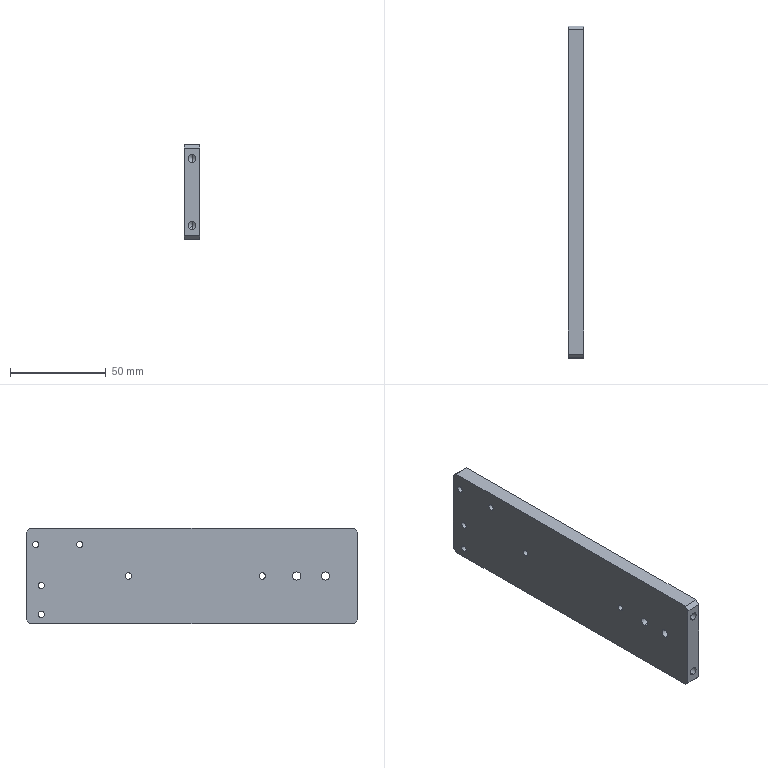Part | STEP file | FBDS-TL-001 | 1 solid | 34 faces | box 8 x 173.5 x 50 mm | volume 68338 mm3 | cylinder 20 | plane 10 | cone 4 | commonest cylinder face diameters 3.3 x12 4.2 x4 4.3 x4
STEP:
#1=CARTESIAN_POINT('',(0.,32.,27.15));
#2=VERTEX_POINT('',#1);
#3=CARTESIAN_POINT('',(0.,32.,22.85));
#4=VERTEX_POINT('',#3);
#5=CARTESIAN_POINT('',(0.,32.,25.));
#6=DIRECTION('',(1.,0.,0.));
#7=DIRECTION('',(0.,0.,-1.));
#8=AXIS2_PLACEMENT_3D('',#5,#6,#7);
#9=CIRCLE('',#8,2.15);
#10=EDGE_CURVE('',#2,#4,#9,.T.);
#11=ORIENTED_EDGE('',*,*,#10,.F.);
#12=CARTESIAN_POINT('',(8.,32.,27.15));
#13=VERTEX_POINT('',#12);
#14=CARTESIAN_POINT('',(8.,32.,27.15));
#15=DIRECTION('',(1.,0.,0.));
#16=VECTOR('',#15,1000.);
#17=LINE('',#14,#16);
#18=EDGE_CURVE('',#2,#13,#17,.T.);
#19=ORIENTED_EDGE('',*,*,#18,.T.);
#20=CARTESIAN_POINT('',(8.,32.,22.85));
#21=VERTEX_POINT('',#20);
#22=CARTESIAN_POINT('',(8.,32.,25.));
#23=DIRECTION('',(1.,0.,0.));
#24=DIRECTION('',(0.,0.,-1.));
#25=AXIS2_PLACEMENT_3D('',#22,#23,#24);
#26=CIRCLE('',#25,2.15);
#27=EDGE_CURVE('',#13,#21,#26,.T.);
#28=ORIENTED_EDGE('',*,*,#27,.T.);
#29=CARTESIAN_POINT('',(8.,32.,22.85));
#30=DIRECTION('',(1.,0.,0.));
#31=VECTOR('',#30,1000.);
#32=LINE('',#29,#31);
#33=EDGE_CURVE('',#4,#21,#32,.T.);
#34=ORIENTED_EDGE('',*,*,#33,.F.);
#35=EDGE_LOOP('',(#11,#19,#28,#34));
#36=FACE_OUTER_BOUND('',#35,.T.);
#37=CARTESIAN_POINT('',(8.,32.,25.));
#38=DIRECTION('',(1.,0.,0.));
#39=DIRECTION('',(0.,0.,-1.));
#40=AXIS2_PLACEMENT_3D('',#37,#38,#39);
#41=CYLINDRICAL_SURFACE('',#40,2.15);
#42=ADVANCED_FACE('',(#36),#41,.F.);
#43=CARTESIAN_POINT('',(0.,17.,27.15));
#44=VERTEX_POINT('',#43);
#45=CARTESIAN_POINT('',(0.,17.,22.85));
#46=VERTEX_POINT('',#45);
#47=CARTESIAN_POINT('',(0.,17.,25.));
#48=DIRECTION('',(1.,0.,0.));
#49=DIRECTION('',(0.,0.,-1.));
#50=AXIS2_PLACEMENT_3D('',#47,#48,#49);
#51=CIRCLE('',#50,2.15);
#52=EDGE_CURVE('',#44,#46,#51,.T.);
#53=ORIENTED_EDGE('',*,*,#52,.F.);
#54=CARTESIAN_POINT('',(8.,17.,27.15));
#55=VERTEX_POINT('',#54);
#56=CARTESIAN_POINT('',(8.,17.,27.15));
#57=DIRECTION('',(1.,0.,0.));
#58=VECTOR('',#57,1000.);
#59=LINE('',#56,#58);
#60=EDGE_CURVE('',#44,#55,#59,.T.);
#61=ORIENTED_EDGE('',*,*,#60,.T.);
#62=CARTESIAN_POINT('',(8.,17.,22.85));
#63=VERTEX_POINT('',#62);
#64=CARTESIAN_POINT('',(8.,17.,25.));
#65=DIRECTION('',(1.,0.,0.));
#66=DIRECTION('',(0.,0.,-1.));
#67=AXIS2_PLACEMENT_3D('',#64,#65,#66);
#68=CIRCLE('',#67,2.15);
#69=EDGE_CURVE('',#55,#63,#68,.T.);
#70=ORIENTED_EDGE('',*,*,#69,.T.);
#71=CARTESIAN_POINT('',(8.,17.,22.85));
#72=DIRECTION('',(1.,0.,0.));
#73=VECTOR('',#72,1000.);
#74=LINE('',#71,#73);
#75=EDGE_CURVE('',#46,#63,#74,.T.);
#76=ORIENTED_EDGE('',*,*,#75,.F.);
#77=EDGE_LOOP('',(#53,#61,#70,#76));
#78=FACE_OUTER_BOUND('',#77,.T.);
#79=CARTESIAN_POINT('',(8.,17.,25.));
#80=DIRECTION('',(1.,0.,0.));
#81=DIRECTION('',(0.,0.,-1.));
#82=AXIS2_PLACEMENT_3D('',#79,#80,#81);
#83=CYLINDRICAL_SURFACE('',#82,2.15);
#84=ADVANCED_FACE('',(#78),#83,.F.);
#85=CARTESIAN_POINT('',(0.,120.,26.65));
#86=VERTEX_POINT('',#85);
#87=CARTESIAN_POINT('',(0.,120.,23.35));
#88=VERTEX_POINT('',#87);
#89=CARTESIAN_POINT('',(0.,120.,25.));
#90=DIRECTION('',(1.,0.,0.));
#91=DIRECTION('',(0.,0.,-1.));
#92=AXIS2_PLACEMENT_3D('',#89,#90,#91);
#93=CIRCLE('',#92,1.65);
#94=EDGE_CURVE('',#86,#88,#93,.T.);
#95=ORIENTED_EDGE('',*,*,#94,.F.);
#96=CARTESIAN_POINT('',(8.,120.,26.65));
#97=VERTEX_POINT('',#96);
#98=CARTESIAN_POINT('',(8.,120.,26.65));
#99=DIRECTION('',(1.,0.,0.));
#100=VECTOR('',#99,1000.);
#101=LINE('',#98,#100);
#102=EDGE_CURVE('',#86,#97,#101,.T.);
#103=ORIENTED_EDGE('',*,*,#102,.T.);
#104=CARTESIAN_POINT('',(8.,120.,23.35));
#105=VERTEX_POINT('',#104);
#106=CARTESIAN_POINT('',(8.,120.,25.));
#107=DIRECTION('',(1.,0.,0.));
#108=DIRECTION('',(0.,0.,-1.));
#109=AXIS2_PLACEMENT_3D('',#106,#107,#108);
#110=CIRCLE('',#109,1.65);
#111=EDGE_CURVE('',#97,#105,#110,.T.);
#112=ORIENTED_EDGE('',*,*,#111,.T.);
#113=CARTESIAN_POINT('',(8.,120.,23.35));
#114=DIRECTION('',(1.,0.,0.));
#115=VECTOR('',#114,1000.);
#116=LINE('',#113,#115);
#117=EDGE_CURVE('',#88,#105,#116,.T.);
#118=ORIENTED_EDGE('',*,*,#117,.F.);
#119=EDGE_LOOP('',(#95,#103,#112,#118));
#120=FACE_OUTER_BOUND('',#119,.T.);
#121=CARTESIAN_POINT('',(8.,120.,25.));
#122=DIRECTION('',(1.,0.,0.));
#123=DIRECTION('',(0.,0.,-1.));
#124=AXIS2_PLACEMENT_3D('',#121,#122,#123);
#125=CYLINDRICAL_SURFACE('',#124,1.65);
#126=ADVANCED_FACE('',(#120),#125,.F.);
#127=CARTESIAN_POINT('',(0.,50.,26.65));
#128=VERTEX_POINT('',#127);
#129=CARTESIAN_POINT('',(0.,50.,23.35));
#130=VERTEX_POINT('',#129);
#131=CARTESIAN_POINT('',(0.,50.,25.));
#132=DIRECTION('',(1.,0.,0.));
#133=DIRECTION('',(0.,0.,-1.));
#134=AXIS2_PLACEMENT_3D('',#131,#132,#133);
#135=CIRCLE('',#134,1.65);
#136=EDGE_CURVE('',#128,#130,#135,.T.);
#137=ORIENTED_EDGE('',*,*,#136,.F.);
#138=CARTESIAN_POINT('',(8.,50.,26.65));
#139=VERTEX_POINT('',#138);
#140=CARTESIAN_POINT('',(8.,50.,26.65));
#141=DIRECTION('',(1.,0.,0.));
#142=VECTOR('',#141,1000.);
#143=LINE('',#140,#142);
#144=EDGE_CURVE('',#128,#139,#143,.T.);
#145=ORIENTED_EDGE('',*,*,#144,.T.);
#146=CARTESIAN_POINT('',(8.,50.,23.35));
#147=VERTEX_POINT('',#146);
#148=CARTESIAN_POINT('',(8.,50.,25.));
#149=DIRECTION('',(1.,0.,0.));
#150=DIRECTION('',(0.,0.,-1.));
#151=AXIS2_PLACEMENT_3D('',#148,#149,#150);
#152=CIRCLE('',#151,1.65);
#153=EDGE_CURVE('',#139,#147,#152,.T.);
#154=ORIENTED_EDGE('',*,*,#153,.T.);
#155=CARTESIAN_POINT('',(8.,50.,23.35));
#156=DIRECTION('',(1.,0.,0.));
#157=VECTOR('',#156,1000.);
#158=LINE('',#155,#157);
#159=EDGE_CURVE('',#130,#147,#158,.T.);
#160=ORIENTED_EDGE('',*,*,#159,.F.);
#161=EDGE_LOOP('',(#137,#145,#154,#160));
#162=FACE_OUTER_BOUND('',#161,.T.);
#163=CARTESIAN_POINT('',(8.,50.,25.));
#164=DIRECTION('',(1.,0.,0.));
#165=DIRECTION('',(0.,0.,-1.));
#166=AXIS2_PLACEMENT_3D('',#163,#164,#165);
#167=CYLINDRICAL_SURFACE('',#166,1.65);
#168=ADVANCED_FACE('',(#162),#167,.F.);
#169=CARTESIAN_POINT('',(8.,165.5,18.35));
#170=VERTEX_POINT('',#169);
#171=CARTESIAN_POINT('',(8.,165.5,21.65));
#172=VERTEX_POINT('',#171);
#173=CARTESIAN_POINT('',(8.,165.5,20.));
#174=DIRECTION('',(-1.,0.,0.));
#175=DIRECTION('',(0.,-1.,0.));
#176=AXIS2_PLACEMENT_3D('',#173,#174,#175);
#177=CIRCLE('',#176,1.65);
#178=EDGE_CURVE('',#170,#172,#177,.T.);
#179=ORIENTED_EDGE('',*,*,#178,.F.);
#180=CARTESIAN_POINT('',(0.,165.5,18.35));
#181=VERTEX_POINT('',#180);
#182=CARTESIAN_POINT('',(0.,165.5,18.35));
#183=DIRECTION('',(-1.,0.,0.));
#184=VECTOR('',#183,1000.);
#185=LINE('',#182,#184);
#186=EDGE_CURVE('',#170,#181,#185,.T.);
#187=ORIENTED_EDGE('',*,*,#186,.T.);
#188=CARTESIAN_POINT('',(0.,165.5,21.65));
#189=VERTEX_POINT('',#188);
#190=CARTESIAN_POINT('',(0.,165.5,20.));
#191=DIRECTION('',(-1.,0.,0.));
#192=DIRECTION('',(0.,0.,1.));
#193=AXIS2_PLACEMENT_3D('',#190,#191,#192);
#194=CIRCLE('',#193,1.65);
#195=EDGE_CURVE('',#181,#189,#194,.T.);
#196=ORIENTED_EDGE('',*,*,#195,.T.);
#197=CARTESIAN_POINT('',(0.,165.5,21.65));
#198=DIRECTION('',(-1.,0.,0.));
#199=VECTOR('',#198,1000.);
#200=LINE('',#197,#199);
#201=EDGE_CURVE('',#172,#189,#200,.T.);
#202=ORIENTED_EDGE('',*,*,#201,.F.);
#203=EDGE_LOOP('',(#179,#187,#196,#202));
#204=FACE_OUTER_BOUND('',#203,.T.);
#205=CARTESIAN_POINT('',(0.,165.5,20.));
#206=DIRECTION('',(-1.,0.,0.));
#207=DIRECTION('',(0.,0.,1.));
#208=AXIS2_PLACEMENT_3D('',#205,#206,#207);
#209=CYLINDRICAL_SURFACE('',#208,1.65);
#210=ADVANCED_FACE('',(#204),#209,.F.);
#211=CARTESIAN_POINT('',(8.,165.5,3.35));
#212=VERTEX_POINT('',#211);
#213=CARTESIAN_POINT('',(8.,165.5,6.65));
#214=VERTEX_POINT('',#213);
#215=CARTESIAN_POINT('',(8.,165.5,5.));
#216=DIRECTION('',(-1.,0.,0.));
#217=DIRECTION('',(0.,-1.,0.));
#218=AXIS2_PLACEMENT_3D('',#215,#216,#217);
#219=CIRCLE('',#218,1.65);
#220=EDGE_CURVE('',#212,#214,#219,.T.);
#221=ORIENTED_EDGE('',*,*,#220,.F.);
#222=CARTESIAN_POINT('',(0.,165.5,3.35));
#223=VERTEX_POINT('',#222);
#224=CARTESIAN_POINT('',(0.,165.5,3.35));
#225=DIRECTION('',(-1.,0.,0.));
#226=VECTOR('',#225,1000.);
#227=LINE('',#224,#226);
#228=EDGE_CURVE('',#212,#223,#227,.T.);
#229=ORIENTED_EDGE('',*,*,#228,.T.);
#230=CARTESIAN_POINT('',(0.,165.5,6.65));
#231=VERTEX_POINT('',#230);
#232=CARTESIAN_POINT('',(0.,165.5,5.));
#233=DIRECTION('',(-1.,0.,0.));
#234=DIRECTION('',(0.,0.,1.));
#235=AXIS2_PLACEMENT_3D('',#232,#233,#234);
#236=CIRCLE('',#235,1.65);
#237=EDGE_CURVE('',#223,#231,#236,.T.);
#238=ORIENTED_EDGE('',*,*,#237,.T.);
#239=CARTESIAN_POINT('',(0.,165.5,6.65));
#240=DIRECTION('',(-1.,0.,0.));
#241=VECTOR('',#240,1000.);
#242=LINE('',#239,#241);
#243=EDGE_CURVE('',#214,#231,#242,.T.);
#244=ORIENTED_EDGE('',*,*,#243,.F.);
#245=EDGE_LOOP('',(#221,#229,#238,#244));
#246=FACE_OUTER_BOUND('',#245,.T.);
#247=CARTESIAN_POINT('',(0.,165.5,5.));
#248=DIRECTION('',(-1.,0.,0.));
#249=DIRECTION('',(0.,0.,1.));
#250=AXIS2_PLACEMENT_3D('',#247,#248,#249);
#251=CYLINDRICAL_SURFACE('',#250,1.65);
#252=ADVANCED_FACE('',(#246),#251,.F.);
#253=CARTESIAN_POINT('',(4.,12.4,9.6));
#254=VERTEX_POINT('',#253);
#255=CARTESIAN_POINT('',(4.,12.4,5.4));
#256=VERTEX_POINT('',#255);
#257=CARTESIAN_POINT('',(4.,12.4,7.5));
#258=DIRECTION('',(0.,-1.,0.));
#259=DIRECTION('',(0.,0.,-1.));
#260=AXIS2_PLACEMENT_3D('',#257,#258,#259);
#261=CIRCLE('',#260,2.1);
#262=EDGE_CURVE('',#254,#256,#261,.T.);
#263=ORIENTED_EDGE('',*,*,#262,.F.);
#264=CARTESIAN_POINT('',(4.,0.,9.6));
#265=VERTEX_POINT('',#264);
#266=CARTESIAN_POINT('',(4.,0.,9.6));
#267=DIRECTION('',(0.,-1.,0.));
#268=VECTOR('',#267,1000.);
#269=LINE('',#266,#268);
#270=EDGE_CURVE('',#254,#265,#269,.T.);
#271=ORIENTED_EDGE('',*,*,#270,.T.);
#272=CARTESIAN_POINT('',(4.,0.,5.4));
#273=VERTEX_POINT('',#272);
#274=CARTESIAN_POINT('',(4.,0.,7.5));
#275=DIRECTION('',(0.,-1.,0.));
#276=DIRECTION('',(0.,0.,-1.));
#277=AXIS2_PLACEMENT_3D('',#274,#275,#276);
#278=CIRCLE('',#277,2.1);
#279=EDGE_CURVE('',#265,#273,#278,.T.);
#280=ORIENTED_EDGE('',*,*,#279,.T.);
#281=CARTESIAN_POINT('',(4.,0.,5.4));
#282=DIRECTION('',(0.,-1.,0.));
#283=VECTOR('',#282,1000.);
#284=LINE('',#281,#283);
#285=EDGE_CURVE('',#256,#273,#284,.T.);
#286=ORIENTED_EDGE('',*,*,#285,.F.);
#287=EDGE_LOOP('',(#263,#271,#280,#286));
#288=FACE_OUTER_BOUND('',#287,.T.);
#289=CARTESIAN_POINT('',(4.,0.,7.5));
#290=DIRECTION('',(0.,-1.,0.));
#291=DIRECTION('',(0.,0.,-1.));
#292=AXIS2_PLACEMENT_3D('',#289,#290,#291);
#293=CYLINDRICAL_SURFACE('',#292,2.1);
#294=ADVANCED_FACE('',(#288),#293,.F.);
#295=CARTESIAN_POINT('',(4.,13.662,7.5));
#296=VERTEX_POINT('',#295);
#297=CARTESIAN_POINT('',(4.,12.4,5.4));
#298=DIRECTION('',(0.,-0.515,-0.8572));
#299=VECTOR('',#298,1000.);
#300=LINE('',#297,#299);
#301=EDGE_CURVE('',#296,#256,#300,.T.);
#302=ORIENTED_EDGE('',*,*,#301,.F.);
#303=CARTESIAN_POINT('',(4.,12.4,9.6));
#304=DIRECTION('',(0.,-0.515,0.8572));
#305=VECTOR('',#304,1000.);
#306=LINE('',#303,#305);
#307=EDGE_CURVE('',#296,#254,#306,.T.);
#308=ORIENTED_EDGE('',*,*,#307,.T.);
#309=ORIENTED_EDGE('',*,*,#262,.T.);
#310=EDGE_LOOP('',(#302,#308,#309));
#311=FACE_OUTER_BOUND('',#310,.T.);
#312=CARTESIAN_POINT('',(4.,12.4,7.5));
#313=DIRECTION('',(0.,-1.,0.));
#314=DIRECTION('',(0.,0.,-1.));
#315=AXIS2_PLACEMENT_3D('',#312,#313,#314);
#316=CONICAL_SURFACE('',#315,2.1,1.03);
#317=ADVANCED_FACE('',(#311),#316,.F.);
#318=CARTESIAN_POINT('',(4.,12.4,44.6));
#319=VERTEX_POINT('',#318);
#320=CARTESIAN_POINT('',(4.,12.4,40.4));
#321=VERTEX_POINT('',#320);
#322=CARTESIAN_POINT('',(4.,12.4,42.5));
#323=DIRECTION('',(0.,-1.,0.));
#324=DIRECTION('',(0.,0.,-1.));
#325=AXIS2_PLACEMENT_3D('',#322,#323,#324);
#326=CIRCLE('',#325,2.1);
#327=EDGE_CURVE('',#319,#321,#326,.T.);
#328=ORIENTED_EDGE('',*,*,#327,.F.);
#329=CARTESIAN_POINT('',(4.,0.,44.6));
#330=VERTEX_POINT('',#329);
#331=CARTESIAN_POINT('',(4.,0.,44.6));
#332=DIRECTION('',(0.,-1.,0.));
#333=VECTOR('',#332,1000.);
#334=LINE('',#331,#333);
#335=EDGE_CURVE('',#319,#330,#334,.T.);
#336=ORIENTED_EDGE('',*,*,#335,.T.);
#337=CARTESIAN_POINT('',(4.,0.,40.4));
#338=VERTEX_POINT('',#337);
#339=CARTESIAN_POINT('',(4.,0.,42.5));
#340=DIRECTION('',(0.,-1.,0.));
#341=DIRECTION('',(0.,0.,-1.));
#342=AXIS2_PLACEMENT_3D('',#339,#340,#341);
#343=CIRCLE('',#342,2.1);
#344=EDGE_CURVE('',#330,#338,#343,.T.);
#345=ORIENTED_EDGE('',*,*,#344,.T.);
#346=CARTESIAN_POINT('',(4.,0.,40.4));
#347=DIRECTION('',(0.,-1.,0.));
#348=VECTOR('',#347,1000.);
#349=LINE('',#346,#348);
#350=EDGE_CURVE('',#321,#338,#349,.T.);
#351=ORIENTED_EDGE('',*,*,#350,.F.);
#352=EDGE_LOOP('',(#328,#336,#345,#351));
#353=FACE_OUTER_BOUND('',#352,.T.);
#354=CARTESIAN_POINT('',(4.,0.,42.5));
#355=DIRECTION('',(0.,-1.,0.));
#356=DIRECTION('',(0.,0.,-1.));
#357=AXIS2_PLACEMENT_3D('',#354,#355,#356);
#358=CYLINDRICAL_SURFACE('',#357,2.1);
#359=ADVANCED_FACE('',(#353),#358,.F.);
#360=CARTESIAN_POINT('',(4.,13.662,42.5));
#361=VERTEX_POINT('',#360);
#362=CARTESIAN_POINT('',(4.,12.4,40.4));
#363=DIRECTION('',(0.,-0.515,-0.8572));
#364=VECTOR('',#363,1000.);
#365=LINE('',#362,#364);
#366=EDGE_CURVE('',#361,#321,#365,.T.);
#367=ORIENTED_EDGE('',*,*,#366,.F.);
#368=CARTESIAN_POINT('',(4.,12.4,44.6));
#369=DIRECTION('',(0.,-0.515,0.8572));
#370=VECTOR('',#369,1000.);
#371=LINE('',#368,#370);
#372=EDGE_CURVE('',#361,#319,#371,.T.);
#373=ORIENTED_EDGE('',*,*,#372,.T.);
#374=ORIENTED_EDGE('',*,*,#327,.T.);
#375=EDGE_LOOP('',(#367,#373,#374));
#376=FACE_OUTER_BOUND('',#375,.T.);
#377=CARTESIAN_POINT('',(4.,12.4,42.5));
#378=DIRECTION('',(0.,-1.,0.));
#379=DIRECTION('',(0.,0.,-1.));
#380=AXIS2_PLACEMENT_3D('',#377,#378,#379);
#381=CONICAL_SURFACE('',#380,2.1,1.03);
#382=ADVANCED_FACE('',(#376),#381,.F.);
#383=CARTESIAN_POINT('',(0.,168.5,43.15));
#384=VERTEX_POINT('',#383);
#385=CARTESIAN_POINT('',(0.,168.5,39.85));
#386=VERTEX_POINT('',#385);
#387=CARTESIAN_POINT('',(0.,168.5,41.5));
#388=DIRECTION('',(1.,0.,0.));
#389=DIRECTION('',(0.,0.,-1.));
#390=AXIS2_PLACEMENT_3D('',#387,#388,#389);
#391=CIRCLE('',#390,1.65);
#392=EDGE_CURVE('',#384,#386,#391,.T.);
#393=ORIENTED_EDGE('',*,*,#392,.F.);
#394=CARTESIAN_POINT('',(8.,168.5,43.15));
#395=VERTEX_POINT('',#394);
#396=CARTESIAN_POINT('',(8.,168.5,43.15));
#397=DIRECTION('',(1.,0.,0.));
#398=VECTOR('',#397,1000.);
#399=LINE('',#396,#398);
#400=EDGE_CURVE('',#384,#395,#399,.T.);
#401=ORIENTED_EDGE('',*,*,#400,.T.);
#402=CARTESIAN_POINT('',(8.,168.5,39.85));
#403=VERTEX_POINT('',#402);
#404=CARTESIAN_POINT('',(8.,168.5,41.5));
#405=DIRECTION('',(1.,0.,0.));
#406=DIRECTION('',(0.,0.,-1.));
#407=AXIS2_PLACEMENT_3D('',#404,#405,#406);
#408=CIRCLE('',#407,1.65);
#409=EDGE_CURVE('',#395,#403,#408,.T.);
#410=ORIENTED_EDGE('',*,*,#409,.T.);
#411=CARTESIAN_POINT('',(8.,168.5,39.85));
#412=DIRECTION('',(1.,0.,0.));
#413=VECTOR('',#412,1000.);
#414=LINE('',#411,#413);
#415=EDGE_CURVE('',#386,#403,#414,.T.);
#416=ORIENTED_EDGE('',*,*,#415,.F.);
#417=EDGE_LOOP('',(#393,#401,#410,#416));
#418=FACE_OUTER_BOUND('',#417,.T.);
#419=CARTESIAN_POINT('',(8.,168.5,41.5));
#420=DIRECTION('',(1.,0.,0.));
#421=DIRECTION('',(0.,0.,-1.));
#422=AXIS2_PLACEMENT_3D('',#419,#420,#421);
#423=CYLINDRICAL_SURFACE('',#422,1.65);
#424=ADVANCED_FACE('',(#418),#423,.F.);
#425=CARTESIAN_POINT('',(0.,145.5,43.15));
#426=VERTEX_POINT('',#425);
#427=CARTESIAN_POINT('',(0.,145.5,39.85));
#428=VERTEX_POINT('',#427);
#429=CARTESIAN_POINT('',(0.,145.5,41.5));
#430=DIRECTION('',(1.,0.,0.));
#431=DIRECTION('',(0.,0.,-1.));
#432=AXIS2_PLACEMENT_3D('',#429,#430,#431);
#433=CIRCLE('',#432,1.65);
#434=EDGE_CURVE('',#426,#428,#433,.T.);
#435=ORIENTED_EDGE('',*,*,#434,.F.);
#436=CARTESIAN_POINT('',(8.,145.5,43.15));
#437=VERTEX_POINT('',#436);
#438=CARTESIAN_POINT('',(8.,145.5,43.15));
#439=DIRECTION('',(1.,0.,0.));
#440=VECTOR('',#439,1000.);
#441=LINE('',#438,#440);
#442=EDGE_CURVE('',#426,#437,#441,.T.);
#443=ORIENTED_EDGE('',*,*,#442,.T.);
#444=CARTESIAN_POINT('',(8.,145.5,39.85));
#445=VERTEX_POINT('',#444);
#446=CARTESIAN_POINT('',(8.,145.5,41.5));
#447=DIRECTION('',(1.,0.,0.));
#448=DIRECTION('',(0.,0.,-1.));
#449=AXIS2_PLACEMENT_3D('',#446,#447,#448);
#450=CIRCLE('',#449,1.65);
#451=EDGE_CURVE('',#437,#445,#450,.T.);
#452=ORIENTED_EDGE('',*,*,#451,.T.);
#453=CARTESIAN_POINT('',(8.,145.5,39.85));
#454=DIRECTION('',(1.,0.,0.));
#455=VECTOR('',#454,1000.);
#456=LINE('',#453,#455);
#457=EDGE_CURVE('',#428,#445,#456,.T.);
#458=ORIENTED_EDGE('',*,*,#457,.F.);
#459=EDGE_LOOP('',(#435,#443,#452,#458));
#460=FACE_OUTER_BOUND('',#459,.T.);
#461=CARTESIAN_POINT('',(8.,145.5,41.5));
#462=DIRECTION('',(1.,0.,0.));
#463=DIRECTION('',(0.,0.,-1.));
#464=AXIS2_PLACEMENT_3D('',#461,#462,#463);
#465=CYLINDRICAL_SURFACE('',#464,1.65);
#466=ADVANCED_FACE('',(#460),#465,.F.);
#467=CARTESIAN_POINT('',(4.,0.,7.5));
#468=DIRECTION('',(0.,-1.,0.));
#469=DIRECTION('',(0.,0.,-1.));
#470=AXIS2_PLACEMENT_3D('',#467,#468,#469);
#471=CIRCLE('',#470,2.1);
#472=EDGE_CURVE('',#273,#265,#471,.T.);
#473=ORIENTED_EDGE('',*,*,#472,.F.);
#474=ORIENTED_EDGE('',*,*,#279,.F.);
#475=EDGE_LOOP('',(#473,#474));
#476=FACE_BOUND('',#475,.T.);
#477=CARTESIAN_POINT('',(4.,0.,42.5));
#478=DIRECTION('',(0.,-1.,0.));
#479=DIRECTION('',(0.,0.,-1.));
#480=AXIS2_PLACEMENT_3D('',#477,#478,#479);
#481=CIRCLE('',#480,2.1);
#482=EDGE_CURVE('',#338,#330,#481,.T.);
#483=ORIENTED_EDGE('',*,*,#482,.F.);
#484=ORIENTED_EDGE('',*,*,#344,.F.);
#485=EDGE_LOOP('',(#483,#484));
#486=FACE_BOUND('',#485,.T.);
#487=CARTESIAN_POINT('',(8.,0.,48.));
#488=VERTEX_POINT('',#487);
#489=CARTESIAN_POINT('',(8.,0.,2.));
#490=VERTEX_POINT('',#489);
#491=CARTESIAN_POINT('',(8.,0.,50.));
#492=DIRECTION('',(0.,0.,-1.));
#493=VECTOR('',#492,1000.);
#494=LINE('',#491,#493);
#495=EDGE_CURVE('',#488,#490,#494,.T.);
#496=ORIENTED_EDGE('',*,*,#495,.F.);
#497=CARTESIAN_POINT('',(0.,0.,48.));
#498=VERTEX_POINT('',#497);
#499=CARTESIAN_POINT('',(8.,0.,48.));
#500=DIRECTION('',(-1.,0.,0.));
#501=VECTOR('',#500,1000.);
#502=LINE('',#499,#501);
#503=EDGE_CURVE('',#488,#498,#502,.T.);
#504=ORIENTED_EDGE('',*,*,#503,.T.);
#505=CARTESIAN_POINT('',(0.,0.,2.));
#506=VERTEX_POINT('',#505);
#507=CARTESIAN_POINT('',(0.,0.,50.));
#508=DIRECTION('',(0.,0.,-1.));
#509=VECTOR('',#508,1000.);
#510=LINE('',#507,#509);
#511=EDGE_CURVE('',#498,#506,#510,.T.);
#512=ORIENTED_EDGE('',*,*,#511,.T.);
#513=CARTESIAN_POINT('',(8.,0.,2.));
#514=DIRECTION('',(1.,0.,0.));
#515=VECTOR('',#514,1000.);
#516=LINE('',#513,#515);
#517=EDGE_CURVE('',#506,#490,#516,.T.);
#518=ORIENTED_EDGE('',*,*,#517,.T.);
#519=EDGE_LOOP('',(#496,#504,#512,#518));
#520=FACE_OUTER_BOUND('',#519,.T.);
#521=CARTESIAN_POINT('',(8.,0.,50.));
#522=DIRECTION('',(0.,1.,0.));
#523=DIRECTION('',(-1.,0.,0.));
#524=AXIS2_PLACEMENT_3D('',#521,#522,#523);
#525=PLANE('',#524);
#526=ADVANCED_FACE('',(#476,#486,#520),#525,.F.);
#527=CARTESIAN_POINT('',(8.,32.,25.));
#528=DIRECTION('',(1.,0.,0.));
#529=DIRECTION('',(0.,0.,-1.));
#530=AXIS2_PLACEMENT_3D('',#527,#528,#529);
#531=CIRCLE('',#530,2.15);
#532=EDGE_CURVE('',#21,#13,#531,.T.);
#533=ORIENTED_EDGE('',*,*,#532,.F.);
#534=ORIENTED_EDGE('',*,*,#27,.F.);
#535=EDGE_LOOP('',(#533,#534));
#536=FACE_BOUND('',#535,.T.);
#537=CARTESIAN_POINT('',(8.,17.,25.));
#538=DIRECTION('',(1.,0.,0.));
#539=DIRECTION('',(0.,0.,-1.));
#540=AXIS2_PLACEMENT_3D('',#537,#538,#539);
#541=CIRCLE('',#540,2.15);
#542=EDGE_CURVE('',#63,#55,#541,.T.);
#543=ORIENTED_EDGE('',*,*,#542,.F.);
#544=ORIENTED_EDGE('',*,*,#69,.F.);
#545=EDGE_LOOP('',(#543,#544));
#546=FACE_BOUND('',#545,.T.);
#547=CARTESIAN_POINT('',(8.,120.,25.));
#548=DIRECTION('',(1.,0.,0.));
#549=DIRECTION('',(0.,0.,-1.));
#550=AXIS2_PLACEMENT_3D('',#547,#548,#549);
#551=CIRCLE('',#550,1.65);
#552=EDGE_CURVE('',#105,#97,#551,.T.);
#553=ORIENTED_EDGE('',*,*,#552,.F.);
#554=ORIENTED_EDGE('',*,*,#111,.F.);
#555=EDGE_LOOP('',(#553,#554));
#556=FACE_BOUND('',#555,.T.);
#557=CARTESIAN_POINT('',(8.,50.,25.));
#558=DIRECTION('',(1.,0.,0.));
#559=DIRECTION('',(0.,0.,-1.));
#560=AXIS2_PLACEMENT_3D('',#557,#558,#559);
#561=CIRCLE('',#560,1.65);
#562=EDGE_CURVE('',#147,#139,#561,.T.);
#563=ORIENTED_EDGE('',*,*,#562,.F.);
#564=ORIENTED_EDGE('',*,*,#153,.F.);
#565=EDGE_LOOP('',(#563,#564));
#566=FACE_BOUND('',#565,.T.);
#567=CARTESIAN_POINT('',(8.,165.5,20.));
#568=DIRECTION('',(-1.,0.,0.));
#569=DIRECTION('',(0.,-1.,0.));
#570=AXIS2_PLACEMENT_3D('',#567,#568,#569);
#571=CIRCLE('',#570,1.65);
#572=EDGE_CURVE('',#172,#170,#571,.T.);
#573=ORIENTED_EDGE('',*,*,#572,.T.);
#574=ORIENTED_EDGE('',*,*,#178,.T.);
#575=EDGE_LOOP('',(#573,#574));
#576=FACE_BOUND('',#575,.T.);
#577=CARTESIAN_POINT('',(8.,165.5,5.));
#578=DIRECTION('',(-1.,0.,0.));
#579=DIRECTION('',(0.,-1.,0.));
#580=AXIS2_PLACEMENT_3D('',#577,#578,#579);
#581=CIRCLE('',#580,1.65);
#582=EDGE_CURVE('',#214,#212,#581,.T.);
#583=ORIENTED_EDGE('',*,*,#582,.T.);
#584=ORIENTED_EDGE('',*,*,#220,.T.);
#585=EDGE_LOOP('',(#583,#584));
#586=FACE_BOUND('',#585,.T.);
#587=CARTESIAN_POINT('',(8.,168.5,41.5));
#588=DIRECTION('',(1.,0.,0.));
#589=DIRECTION('',(0.,0.,-1.));
#590=AXIS2_PLACEMENT_3D('',#587,#588,#589);
#591=CIRCLE('',#590,1.65);
#592=EDGE_CURVE('',#403,#395,#591,.T.);
#593=ORIENTED_EDGE('',*,*,#592,.F.);
#594=ORIENTED_EDGE('',*,*,#409,.F.);
#595=EDGE_LOOP('',(#593,#594));
#596=FACE_BOUND('',#595,.T.);
#597=CARTESIAN_POINT('',(8.,145.5,41.5));
#598=DIRECTION('',(1.,0.,0.));
#599=DIRECTION('',(0.,0.,-1.));
#600=AXIS2_PLACEMENT_3D('',#597,#598,#599);
#601=CIRCLE('',#600,1.65);
#602=EDGE_CURVE('',#445,#437,#601,.T.);
#603=ORIENTED_EDGE('',*,*,#602,.F.);
#604=ORIENTED_EDGE('',*,*,#451,.F.);
#605=EDGE_LOOP('',(#603,#604));
#606=FACE_BOUND('',#605,.T.);
#607=CARTESIAN_POINT('',(8.,2.,50.));
#608=VERTEX_POINT('',#607);
#609=CARTESIAN_POINT('',(8.,171.5,50.));
#610=VERTEX_POINT('',#609);
#611=CARTESIAN_POINT('',(8.,173.5,50.));
#612=DIRECTION('',(0.,1.,0.));
#613=VECTOR('',#612,1000.);
#614=LINE('',#611,#613);
#615=EDGE_CURVE('',#608,#610,#614,.T.);
#616=ORIENTED_EDGE('',*,*,#615,.F.);
#617=CARTESIAN_POINT('',(8.,2.,50.));
#618=DIRECTION('',(0.,-0.7071,-0.7071));
#619=VECTOR('',#618,1000.);
#620=LINE('',#617,#619);
#621=EDGE_CURVE('',#608,#488,#620,.T.);
#622=ORIENTED_EDGE('',*,*,#621,.T.);
#623=ORIENTED_EDGE('',*,*,#495,.T.);
#624=CARTESIAN_POINT('',(8.,2.,0.));
#625=VERTEX_POINT('',#624);
#626=CARTESIAN_POINT('',(8.,0.,2.));
#627=DIRECTION('',(0.,0.7071,-0.7071));
#628=VECTOR('',#627,1000.);
#629=LINE('',#626,#628);
#630=EDGE_CURVE('',#490,#625,#629,.T.);
#631=ORIENTED_EDGE('',*,*,#630,.T.);
#632=CARTESIAN_POINT('',(8.,171.5,0.));
#633=VERTEX_POINT('',#632);
#634=CARTESIAN_POINT('',(8.,173.5,0.));
#635=DIRECTION('',(0.,1.,0.));
#636=VECTOR('',#635,1000.);
#637=LINE('',#634,#636);
#638=EDGE_CURVE('',#625,#633,#637,.T.);
#639=ORIENTED_EDGE('',*,*,#638,.T.);
#640=CARTESIAN_POINT('',(8.,173.5,2.));
#641=VERTEX_POINT('',#640);
#642=CARTESIAN_POINT('',(8.,173.5,2.));
#643=DIRECTION('',(0.,0.7071,0.7071));
#644=VECTOR('',#643,1000.);
#645=LINE('',#642,#644);
#646=EDGE_CURVE('',#633,#641,#645,.T.);
#647=ORIENTED_EDGE('',*,*,#646,.T.);
#648=CARTESIAN_POINT('',(8.,173.5,48.));
#649=VERTEX_POINT('',#648);
#650=CARTESIAN_POINT('',(8.,173.5,50.));
#651=DIRECTION('',(0.,0.,-1.));
#652=VECTOR('',#651,1000.);
#653=LINE('',#650,#652);
#654=EDGE_CURVE('',#649,#641,#653,.T.);
#655=ORIENTED_EDGE('',*,*,#654,.F.);
#656=CARTESIAN_POINT('',(8.,171.5,50.));
#657=DIRECTION('',(0.,-0.7071,0.7071));
#658=VECTOR('',#657,1000.);
#659=LINE('',#656,#658);
#660=EDGE_CURVE('',#649,#610,#659,.T.);
#661=ORIENTED_EDGE('',*,*,#660,.T.);
#662=EDGE_LOOP('',(#616,#622,#623,#631,#639,#647,#655,#661));
#663=FACE_OUTER_BOUND('',#662,.T.);
#664=CARTESIAN_POINT('',(8.,173.5,50.));
#665=DIRECTION('',(-1.,0.,0.));
#666=DIRECTION('',(0.,-1.,0.));
#667=AXIS2_PLACEMENT_3D('',#664,#665,#666);
#668=PLANE('',#667);
#669=ADVANCED_FACE('',(#536,#546,#556,#566,#576,#586,#596,#606,#663),#668,.F.);
#670=ORIENTED_EDGE('',*,*,#654,.T.);
#671=CARTESIAN_POINT('',(0.,173.5,2.));
#672=VERTEX_POINT('',#671);
#673=CARTESIAN_POINT('',(0.,173.5,2.));
#674=DIRECTION('',(-1.,0.,0.));
#675=VECTOR('',#674,1000.);
#676=LINE('',#673,#675);
#677=EDGE_CURVE('',#641,#672,#676,.T.);
#678=ORIENTED_EDGE('',*,*,#677,.T.);
#679=CARTESIAN_POINT('',(0.,173.5,48.));
#680=VERTEX_POINT('',#679);
#681=CARTESIAN_POINT('',(0.,173.5,50.));
#682=DIRECTION('',(0.,0.,-1.));
#683=VECTOR('',#682,1000.);
#684=LINE('',#681,#683);
#685=EDGE_CURVE('',#680,#672,#684,.T.);
#686=ORIENTED_EDGE('',*,*,#685,.F.);
#687=CARTESIAN_POINT('',(0.,173.5,48.));
#688=DIRECTION('',(1.,0.,0.));
#689=VECTOR('',#688,1000.);
#690=LINE('',#687,#689);
#691=EDGE_CURVE('',#680,#649,#690,.T.);
#692=ORIENTED_EDGE('',*,*,#691,.T.);
#693=EDGE_LOOP('',(#670,#678,#686,#692));
#694=FACE_OUTER_BOUND('',#693,.T.);
#695=CARTESIAN_POINT('',(0.,173.5,50.));
#696=DIRECTION('',(0.,-1.,0.));
#697=DIRECTION('',(0.,0.,-1.));
#698=AXIS2_PLACEMENT_3D('',#695,#696,#697);
#699=PLANE('',#698);
#700=ADVANCED_FACE('',(#694),#699,.F.);
#701=CARTESIAN_POINT('',(0.,32.,25.));
#702=DIRECTION('',(1.,0.,0.));
#703=DIRECTION('',(0.,0.,-1.));
#704=AXIS2_PLACEMENT_3D('',#701,#702,#703);
#705=CIRCLE('',#704,2.15);
#706=EDGE_CURVE('',#4,#2,#705,.T.);
#707=ORIENTED_EDGE('',*,*,#706,.T.);
#708=ORIENTED_EDGE('',*,*,#10,.T.);
#709=EDGE_LOOP('',(#707,#708));
#710=FACE_BOUND('',#709,.T.);
#711=CARTESIAN_POINT('',(0.,17.,25.));
#712=DIRECTION('',(1.,0.,0.));
#713=DIRECTION('',(0.,0.,-1.));
#714=AXIS2_PLACEMENT_3D('',#711,#712,#713);
#715=CIRCLE('',#714,2.15);
#716=EDGE_CURVE('',#46,#44,#715,.T.);
#717=ORIENTED_EDGE('',*,*,#716,.T.);
#718=ORIENTED_EDGE('',*,*,#52,.T.);
#719=EDGE_LOOP('',(#717,#718));
#720=FACE_BOUND('',#719,.T.);
#721=CARTESIAN_POINT('',(0.,120.,25.));
#722=DIRECTION('',(1.,0.,0.));
#723=DIRECTION('',(0.,0.,-1.));
#724=AXIS2_PLACEMENT_3D('',#721,#722,#723);
#725=CIRCLE('',#724,1.65);
#726=EDGE_CURVE('',#88,#86,#725,.T.);
#727=ORIENTED_EDGE('',*,*,#726,.T.);
#728=ORIENTED_EDGE('',*,*,#94,.T.);
#729=EDGE_LOOP('',(#727,#728));
#730=FACE_BOUND('',#729,.T.);
#731=CARTESIAN_POINT('',(0.,50.,25.));
#732=DIRECTION('',(1.,0.,0.));
#733=DIRECTION('',(0.,0.,-1.));
#734=AXIS2_PLACEMENT_3D('',#731,#732,#733);
#735=CIRCLE('',#734,1.65);
#736=EDGE_CURVE('',#130,#128,#735,.T.);
#737=ORIENTED_EDGE('',*,*,#736,.T.);
#738=ORIENTED_EDGE('',*,*,#136,.T.);
#739=EDGE_LOOP('',(#737,#738));
#740=FACE_BOUND('',#739,.T.);
#741=CARTESIAN_POINT('',(0.,165.5,20.));
#742=DIRECTION('',(-1.,0.,0.));
#743=DIRECTION('',(0.,0.,1.));
#744=AXIS2_PLACEMENT_3D('',#741,#742,#743);
#745=CIRCLE('',#744,1.65);
#746=EDGE_CURVE('',#189,#181,#745,.T.);
#747=ORIENTED_EDGE('',*,*,#746,.F.);
#748=ORIENTED_EDGE('',*,*,#195,.F.);
#749=EDGE_LOOP('',(#747,#748));
#750=FACE_BOUND('',#749,.T.);
#751=CARTESIAN_POINT('',(0.,165.5,5.));
#752=DIRECTION('',(-1.,0.,0.));
#753=DIRECTION('',(0.,0.,1.));
#754=AXIS2_PLACEMENT_3D('',#751,#752,#753);
#755=CIRCLE('',#754,1.65);
#756=EDGE_CURVE('',#231,#223,#755,.T.);
#757=ORIENTED_EDGE('',*,*,#756,.F.);
#758=ORIENTED_EDGE('',*,*,#237,.F.);
#759=EDGE_LOOP('',(#757,#758));
#760=FACE_BOUND('',#759,.T.);
#761=CARTESIAN_POINT('',(0.,168.5,41.5));
#762=DIRECTION('',(1.,0.,0.));
#763=DIRECTION('',(0.,0.,-1.));
#764=AXIS2_PLACEMENT_3D('',#761,#762,#763);
#765=CIRCLE('',#764,1.65);
#766=EDGE_CURVE('',#386,#384,#765,.T.);
#767=ORIENTED_EDGE('',*,*,#766,.T.);
#768=ORIENTED_EDGE('',*,*,#392,.T.);
#769=EDGE_LOOP('',(#767,#768));
#770=FACE_BOUND('',#769,.T.);
#771=CARTESIAN_POINT('',(0.,145.5,41.5));
#772=DIRECTION('',(1.,0.,0.));
#773=DIRECTION('',(0.,0.,-1.));
#774=AXIS2_PLACEMENT_3D('',#771,#772,#773);
#775=CIRCLE('',#774,1.65);
#776=EDGE_CURVE('',#428,#426,#775,.T.);
#777=ORIENTED_EDGE('',*,*,#776,.T.);
#778=ORIENTED_EDGE('',*,*,#434,.T.);
#779=EDGE_LOOP('',(#777,#778));
#780=FACE_BOUND('',#779,.T.);
#781=ORIENTED_EDGE('',*,*,#511,.F.);
#782=CARTESIAN_POINT('',(0.,2.,50.));
#783=VERTEX_POINT('',#782);
#784=CARTESIAN_POINT('',(0.,2.,50.));
#785=DIRECTION('',(0.,0.7071,0.7071));
#786=VECTOR('',#785,1000.);
#787=LINE('',#784,#786);
#788=EDGE_CURVE('',#498,#783,#787,.T.);
#789=ORIENTED_EDGE('',*,*,#788,.T.);
#790=CARTESIAN_POINT('',(0.,171.5,50.));
#791=VERTEX_POINT('',#790);
#792=CARTESIAN_POINT('',(0.,0.,50.));
#793=DIRECTION('',(0.,-1.,0.));
#794=VECTOR('',#793,1000.);
#795=LINE('',#792,#794);
#796=EDGE_CURVE('',#791,#783,#795,.T.);
#797=ORIENTED_EDGE('',*,*,#796,.F.);
#798=CARTESIAN_POINT('',(0.,171.5,50.));
#799=DIRECTION('',(0.,0.7071,-0.7071));
#800=VECTOR('',#799,1000.);
#801=LINE('',#798,#800);
#802=EDGE_CURVE('',#791,#680,#801,.T.);
#803=ORIENTED_EDGE('',*,*,#802,.T.);
#804=ORIENTED_EDGE('',*,*,#685,.T.);
#805=CARTESIAN_POINT('',(0.,171.5,0.));
#806=VERTEX_POINT('',#805);
#807=CARTESIAN_POINT('',(0.,173.5,2.));
#808=DIRECTION('',(0.,-0.7071,-0.7071));
#809=VECTOR('',#808,1000.);
#810=LINE('',#807,#809);
#811=EDGE_CURVE('',#672,#806,#810,.T.);
#812=ORIENTED_EDGE('',*,*,#811,.T.);
#813=CARTESIAN_POINT('',(0.,2.,0.));
#814=VERTEX_POINT('',#813);
#815=CARTESIAN_POINT('',(0.,0.,0.));
#816=DIRECTION('',(0.,-1.,0.));
#817=VECTOR('',#816,1000.);
#818=LINE('',#815,#817);
#819=EDGE_CURVE('',#806,#814,#818,.T.);
#820=ORIENTED_EDGE('',*,*,#819,.T.);
#821=CARTESIAN_POINT('',(0.,0.,2.));
#822=DIRECTION('',(0.,-0.7071,0.7071));
#823=VECTOR('',#822,1000.);
#824=LINE('',#821,#823);
#825=EDGE_CURVE('',#814,#506,#824,.T.);
#826=ORIENTED_EDGE('',*,*,#825,.T.);
#827=EDGE_LOOP('',(#781,#789,#797,#803,#804,#812,#820,#826));
#828=FACE_OUTER_BOUND('',#827,.T.);
#829=CARTESIAN_POINT('',(0.,0.,50.));
#830=DIRECTION('',(1.,0.,0.));
#831=DIRECTION('',(0.,0.,-1.));
#832=AXIS2_PLACEMENT_3D('',#829,#830,#831);
#833=PLANE('',#832);
#834=ADVANCED_FACE('',(#710,#720,#730,#740,#750,#760,#770,#780,#828),#833,.F.);
#835=ORIENTED_EDGE('',*,*,#796,.T.);
#836=CARTESIAN_POINT('',(0.,2.,50.));
#837=DIRECTION('',(1.,0.,0.));
#838=VECTOR('',#837,1000.);
#839=LINE('',#836,#838);
#840=EDGE_CURVE('',#783,#608,#839,.T.);
#841=ORIENTED_EDGE('',*,*,#840,.T.);
#842=ORIENTED_EDGE('',*,*,#615,.T.);
#843=CARTESIAN_POINT('',(0.,171.5,50.));
#844=DIRECTION('',(-1.,0.,0.));
#845=VECTOR('',#844,1000.);
#846=LINE('',#843,#845);
#847=EDGE_CURVE('',#610,#791,#846,.T.);
#848=ORIENTED_EDGE('',*,*,#847,.T.);
#849=EDGE_LOOP('',(#835,#841,#842,#848));
#850=FACE_OUTER_BOUND('',#849,.T.);
#851=CARTESIAN_POINT('',(0.,0.,50.));
#852=DIRECTION('',(0.,0.,-1.));
#853=DIRECTION('',(-1.,0.,0.));
#854=AXIS2_PLACEMENT_3D('',#851,#852,#853);
#855=PLANE('',#854);
#856=ADVANCED_FACE('',(#850),#855,.F.);
#857=ORIENTED_EDGE('',*,*,#638,.F.);
#858=CARTESIAN_POINT('',(0.,2.,0.));
#859=DIRECTION('',(-1.,0.,0.));
#860=VECTOR('',#859,1000.);
#861=LINE('',#858,#860);
#862=EDGE_CURVE('',#625,#814,#861,.T.);
#863=ORIENTED_EDGE('',*,*,#862,.T.);
#864=ORIENTED_EDGE('',*,*,#819,.F.);
#865=CARTESIAN_POINT('',(8.,171.5,0.));
#866=DIRECTION('',(1.,0.,0.));
#867=VECTOR('',#866,1000.);
#868=LINE('',#865,#867);
#869=EDGE_CURVE('',#806,#633,#868,.T.);
#870=ORIENTED_EDGE('',*,*,#869,.T.);
#871=EDGE_LOOP('',(#857,#863,#864,#870));
#872=FACE_OUTER_BOUND('',#871,.T.);
#873=CARTESIAN_POINT('',(0.,0.,0.));
#874=DIRECTION('',(0.,0.,-1.));
#875=DIRECTION('',(-1.,0.,0.));
#876=AXIS2_PLACEMENT_3D('',#873,#874,#875);
#877=PLANE('',#876);
#878=ADVANCED_FACE('',(#872),#877,.T.);
#879=ORIENTED_EDGE('',*,*,#442,.F.);
#880=ORIENTED_EDGE('',*,*,#776,.F.);
#881=ORIENTED_EDGE('',*,*,#457,.T.);
#882=ORIENTED_EDGE('',*,*,#602,.T.);
#883=EDGE_LOOP('',(#879,#880,#881,#882));
#884=FACE_OUTER_BOUND('',#883,.T.);
#885=CARTESIAN_POINT('',(8.,145.5,41.5));
#886=DIRECTION('',(1.,0.,0.));
#887=DIRECTION('',(0.,0.,-1.));
#888=AXIS2_PLACEMENT_3D('',#885,#886,#887);
#889=CYLINDRICAL_SURFACE('',#888,1.65);
#890=ADVANCED_FACE('',(#884),#889,.F.);
#891=ORIENTED_EDGE('',*,*,#400,.F.);
#892=ORIENTED_EDGE('',*,*,#766,.F.);
#893=ORIENTED_EDGE('',*,*,#415,.T.);
#894=ORIENTED_EDGE('',*,*,#592,.T.);
#895=EDGE_LOOP('',(#891,#892,#893,#894));
#896=FACE_OUTER_BOUND('',#895,.T.);
#897=CARTESIAN_POINT('',(8.,168.5,41.5));
#898=DIRECTION('',(1.,0.,0.));
#899=DIRECTION('',(0.,0.,-1.));
#900=AXIS2_PLACEMENT_3D('',#897,#898,#899);
#901=CYLINDRICAL_SURFACE('',#900,1.65);
#902=ADVANCED_FACE('',(#896),#901,.F.);
#903=ORIENTED_EDGE('',*,*,#372,.F.);
#904=ORIENTED_EDGE('',*,*,#366,.T.);
#905=CARTESIAN_POINT('',(4.,12.4,42.5));
#906=DIRECTION('',(0.,-1.,0.));
#907=DIRECTION('',(0.,0.,-1.));
#908=AXIS2_PLACEMENT_3D('',#905,#906,#907);
#909=CIRCLE('',#908,2.1);
#910=EDGE_CURVE('',#321,#319,#909,.T.);
#911=ORIENTED_EDGE('',*,*,#910,.T.);
#912=EDGE_LOOP('',(#903,#904,#911));
#913=FACE_OUTER_BOUND('',#912,.T.);
#914=CARTESIAN_POINT('',(4.,12.4,42.5));
#915=DIRECTION('',(0.,-1.,0.));
#916=DIRECTION('',(0.,0.,-1.));
#917=AXIS2_PLACEMENT_3D('',#914,#915,#916);
#918=CONICAL_SURFACE('',#917,2.1,1.03);
#919=ADVANCED_FACE('',(#913),#918,.F.);
#920=ORIENTED_EDGE('',*,*,#335,.F.);
#921=ORIENTED_EDGE('',*,*,#910,.F.);
#922=ORIENTED_EDGE('',*,*,#350,.T.);
#923=ORIENTED_EDGE('',*,*,#482,.T.);
#924=EDGE_LOOP('',(#920,#921,#922,#923));
#925=FACE_OUTER_BOUND('',#924,.T.);
#926=CARTESIAN_POINT('',(4.,0.,42.5));
#927=DIRECTION('',(0.,-1.,0.));
#928=DIRECTION('',(0.,0.,-1.));
#929=AXIS2_PLACEMENT_3D('',#926,#927,#928);
#930=CYLINDRICAL_SURFACE('',#929,2.1);
#931=ADVANCED_FACE('',(#925),#930,.F.);
#932=ORIENTED_EDGE('',*,*,#307,.F.);
#933=ORIENTED_EDGE('',*,*,#301,.T.);
#934=CARTESIAN_POINT('',(4.,12.4,7.5));
#935=DIRECTION('',(0.,-1.,0.));
#936=DIRECTION('',(0.,0.,-1.));
#937=AXIS2_PLACEMENT_3D('',#934,#935,#936);
#938=CIRCLE('',#937,2.1);
#939=EDGE_CURVE('',#256,#254,#938,.T.);
#940=ORIENTED_EDGE('',*,*,#939,.T.);
#941=EDGE_LOOP('',(#932,#933,#940));
#942=FACE_OUTER_BOUND('',#941,.T.);
#943=CARTESIAN_POINT('',(4.,12.4,7.5));
#944=DIRECTION('',(0.,-1.,0.));
#945=DIRECTION('',(0.,0.,-1.));
#946=AXIS2_PLACEMENT_3D('',#943,#944,#945);
#947=CONICAL_SURFACE('',#946,2.1,1.03);
#948=ADVANCED_FACE('',(#942),#947,.F.);
#949=ORIENTED_EDGE('',*,*,#270,.F.);
#950=ORIENTED_EDGE('',*,*,#939,.F.);
#951=ORIENTED_EDGE('',*,*,#285,.T.);
#952=ORIENTED_EDGE('',*,*,#472,.T.);
#953=EDGE_LOOP('',(#949,#950,#951,#952));
#954=FACE_OUTER_BOUND('',#953,.T.);
#955=CARTESIAN_POINT('',(4.,0.,7.5));
#956=DIRECTION('',(0.,-1.,0.));
#957=DIRECTION('',(0.,0.,-1.));
#958=AXIS2_PLACEMENT_3D('',#955,#956,#957);
#959=CYLINDRICAL_SURFACE('',#958,2.1);
#960=ADVANCED_FACE('',(#954),#959,.F.);
#961=ORIENTED_EDGE('',*,*,#788,.F.);
#962=ORIENTED_EDGE('',*,*,#503,.F.);
#963=ORIENTED_EDGE('',*,*,#621,.F.);
#964=ORIENTED_EDGE('',*,*,#840,.F.);
#965=EDGE_LOOP('',(#961,#962,#963,#964));
#966=FACE_OUTER_BOUND('',#965,.T.);
#967=CARTESIAN_POINT('',(0.,2.,50.));
#968=DIRECTION('',(0.,0.7071,-0.7071));
#969=DIRECTION('',(1.,0.,0.));
#970=AXIS2_PLACEMENT_3D('',#967,#968,#969);
#971=PLANE('',#970);
#972=ADVANCED_FACE('',(#966),#971,.F.);
#973=ORIENTED_EDGE('',*,*,#825,.F.);
#974=ORIENTED_EDGE('',*,*,#862,.F.);
#975=ORIENTED_EDGE('',*,*,#630,.F.);
#976=ORIENTED_EDGE('',*,*,#517,.F.);
#977=EDGE_LOOP('',(#973,#974,#975,#976));
#978=FACE_OUTER_BOUND('',#977,.T.);
#979=CARTESIAN_POINT('',(8.,0.,2.));
#980=DIRECTION('',(0.,-0.7071,-0.7071));
#981=DIRECTION('',(-1.,0.,0.));
#982=AXIS2_PLACEMENT_3D('',#979,#980,#981);
#983=PLANE('',#982);
#984=ADVANCED_FACE('',(#978),#983,.T.);
#985=ORIENTED_EDGE('',*,*,#646,.F.);
#986=ORIENTED_EDGE('',*,*,#869,.F.);
#987=ORIENTED_EDGE('',*,*,#811,.F.);
#988=ORIENTED_EDGE('',*,*,#677,.F.);
#989=EDGE_LOOP('',(#985,#986,#987,#988));
#990=FACE_OUTER_BOUND('',#989,.T.);
#991=CARTESIAN_POINT('',(0.,173.5,2.));
#992=DIRECTION('',(0.,0.7071,-0.7071));
#993=DIRECTION('',(1.,0.,0.));
#994=AXIS2_PLACEMENT_3D('',#991,#992,#993);
#995=PLANE('',#994);
#996=ADVANCED_FACE('',(#990),#995,.T.);
#997=ORIENTED_EDGE('',*,*,#660,.F.);
#998=ORIENTED_EDGE('',*,*,#691,.F.);
#999=ORIENTED_EDGE('',*,*,#802,.F.);
#1000=ORIENTED_EDGE('',*,*,#847,.F.);
#1001=EDGE_LOOP('',(#997,#998,#999,#1000));
#1002=FACE_OUTER_BOUND('',#1001,.T.);
#1003=CARTESIAN_POINT('',(0.,171.5,50.));
#1004=DIRECTION('',(0.,-0.7071,-0.7071));
#1005=DIRECTION('',(-1.,0.,0.));
#1006=AXIS2_PLACEMENT_3D('',#1003,#1004,#1005);
#1007=PLANE('',#1006);
#1008=ADVANCED_FACE('',(#1002),#1007,.F.);
#1009=ORIENTED_EDGE('',*,*,#228,.F.);
#1010=ORIENTED_EDGE('',*,*,#582,.F.);
#1011=ORIENTED_EDGE('',*,*,#243,.T.);
#1012=ORIENTED_EDGE('',*,*,#756,.T.);
#1013=EDGE_LOOP('',(#1009,#1010,#1011,#1012));
#1014=FACE_OUTER_BOUND('',#1013,.T.);
#1015=CARTESIAN_POINT('',(0.,165.5,5.));
#1016=DIRECTION('',(-1.,0.,0.));
#1017=DIRECTION('',(0.,0.,1.));
#1018=AXIS2_PLACEMENT_3D('',#1015,#1016,#1017);
#1019=CYLINDRICAL_SURFACE('',#1018,1.65);
#1020=ADVANCED_FACE('',(#1014),#1019,.F.);
#1021=ORIENTED_EDGE('',*,*,#186,.F.);
#1022=ORIENTED_EDGE('',*,*,#572,.F.);
#1023=ORIENTED_EDGE('',*,*,#201,.T.);
#1024=ORIENTED_EDGE('',*,*,#746,.T.);
#1025=EDGE_LOOP('',(#1021,#1022,#1023,#1024));
#1026=FACE_OUTER_BOUND('',#1025,.T.);
#1027=CARTESIAN_POINT('',(0.,165.5,20.));
#1028=DIRECTION('',(-1.,0.,0.));
#1029=DIRECTION('',(0.,0.,1.));
#1030=AXIS2_PLACEMENT_3D('',#1027,#1028,#1029);
#1031=CYLINDRICAL_SURFACE('',#1030,1.65);
#1032=ADVANCED_FACE('',(#1026),#1031,.F.);
#1033=ORIENTED_EDGE('',*,*,#144,.F.);
#1034=ORIENTED_EDGE('',*,*,#736,.F.);
#1035=ORIENTED_EDGE('',*,*,#159,.T.);
#1036=ORIENTED_EDGE('',*,*,#562,.T.);
#1037=EDGE_LOOP('',(#1033,#1034,#1035,#1036));
#1038=FACE_OUTER_BOUND('',#1037,.T.);
#1039=CARTESIAN_POINT('',(8.,50.,25.));
#1040=DIRECTION('',(1.,0.,0.));
#1041=DIRECTION('',(0.,0.,-1.));
#1042=AXIS2_PLACEMENT_3D('',#1039,#1040,#1041);
#1043=CYLINDRICAL_SURFACE('',#1042,1.65);
#1044=ADVANCED_FACE('',(#1038),#1043,.F.);
#1045=ORIENTED_EDGE('',*,*,#102,.F.);
#1046=ORIENTED_EDGE('',*,*,#726,.F.);
#1047=ORIENTED_EDGE('',*,*,#117,.T.);
#1048=ORIENTED_EDGE('',*,*,#552,.T.);
#1049=EDGE_LOOP('',(#1045,#1046,#1047,#1048));
#1050=FACE_OUTER_BOUND('',#1049,.T.);
#1051=CARTESIAN_POINT('',(8.,120.,25.));
#1052=DIRECTION('',(1.,0.,0.));
#1053=DIRECTION('',(0.,0.,-1.));
#1054=AXIS2_PLACEMENT_3D('',#1051,#1052,#1053);
#1055=CYLINDRICAL_SURFACE('',#1054,1.65);
#1056=ADVANCED_FACE('',(#1050),#1055,.F.);
#1057=ORIENTED_EDGE('',*,*,#60,.F.);
#1058=ORIENTED_EDGE('',*,*,#716,.F.);
#1059=ORIENTED_EDGE('',*,*,#75,.T.);
#1060=ORIENTED_EDGE('',*,*,#542,.T.);
#1061=EDGE_LOOP('',(#1057,#1058,#1059,#1060));
#1062=FACE_OUTER_BOUND('',#1061,.T.);
#1063=CARTESIAN_POINT('',(8.,17.,25.));
#1064=DIRECTION('',(1.,0.,0.));
#1065=DIRECTION('',(0.,0.,-1.));
#1066=AXIS2_PLACEMENT_3D('',#1063,#1064,#1065);
#1067=CYLINDRICAL_SURFACE('',#1066,2.15);
#1068=ADVANCED_FACE('',(#1062),#1067,.F.);
#1069=ORIENTED_EDGE('',*,*,#18,.F.);
#1070=ORIENTED_EDGE('',*,*,#706,.F.);
#1071=ORIENTED_EDGE('',*,*,#33,.T.);
#1072=ORIENTED_EDGE('',*,*,#532,.T.);
#1073=EDGE_LOOP('',(#1069,#1070,#1071,#1072));
#1074=FACE_OUTER_BOUND('',#1073,.T.);
#1075=CARTESIAN_POINT('',(8.,32.,25.));
#1076=DIRECTION('',(1.,0.,0.));
#1077=DIRECTION('',(0.,0.,-1.));
#1078=AXIS2_PLACEMENT_3D('',#1075,#1076,#1077);
#1079=CYLINDRICAL_SURFACE('',#1078,2.15);
#1080=ADVANCED_FACE('',(#1074),#1079,.F.);
#1081=CLOSED_SHELL('',(#42,#84,#126,#168,#210,#252,#294,#317,#359,#382,#424,#466,#526,#669,#700,#834,#856,#878,#890,#902,#919,#931,#948,#960,#972,#984,#996,#1008,#1020,#1032,#1044,#1056,#1068,#1080));
#1082=MANIFOLD_SOLID_BREP('',#1081);
#1083=CARTESIAN_POINT('',(0.,0.,0.));
#1084=DIRECTION('',(0.,0.,1.));
#1085=DIRECTION('',(1.,0.,0.));
#1086=AXIS2_PLACEMENT_3D('',#1083,#1084,#1085);
#1087=(LENGTH_UNIT()NAMED_UNIT(*)SI_UNIT(.MILLI.,.METRE.));
#1088=UNCERTAINTY_MEASURE_WITH_UNIT(LENGTH_MEASURE(0.00001),#1087,'','');
#1089=(NAMED_UNIT(*)PLANE_ANGLE_UNIT()SI_UNIT($,.RADIAN.));
#1090=(NAMED_UNIT(*)SI_UNIT($,.STERADIAN.)SOLID_ANGLE_UNIT());
#1091=(GEOMETRIC_REPRESENTATION_CONTEXT(3)GLOBAL_UNCERTAINTY_ASSIGNED_CONTEXT((#1088))GLOBAL_UNIT_ASSIGNED_CONTEXT((#1087,#1089,#1090))REPRESENTATION_CONTEXT('',''));
#1092=ADVANCED_BREP_SHAPE_REPRESENTATION('',(#1082,#1086),#1091);